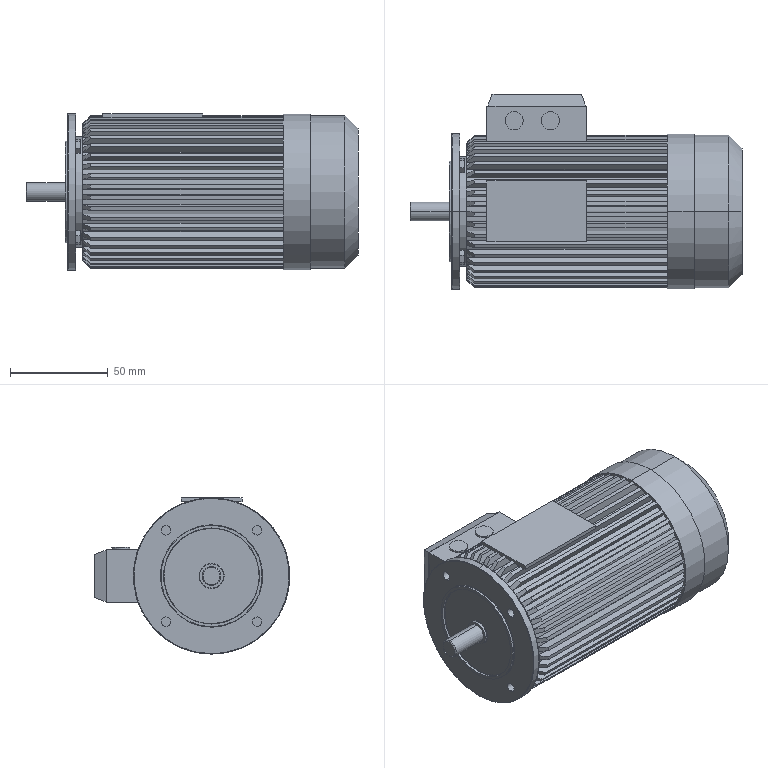Part | STEP file | XB motor_BWED3922_Y_90L.step | 1 solid | 349 faces | box 170 x 100 x 80 mm | volume 524575 mm3 | plane 212 | cylinder 77 | cone 50 | spline 10 | commonest cylinder face diameters 70.2 x47 4.8 x8 9.273 x4 9.6 x2 12.4 x2 49.2 x2